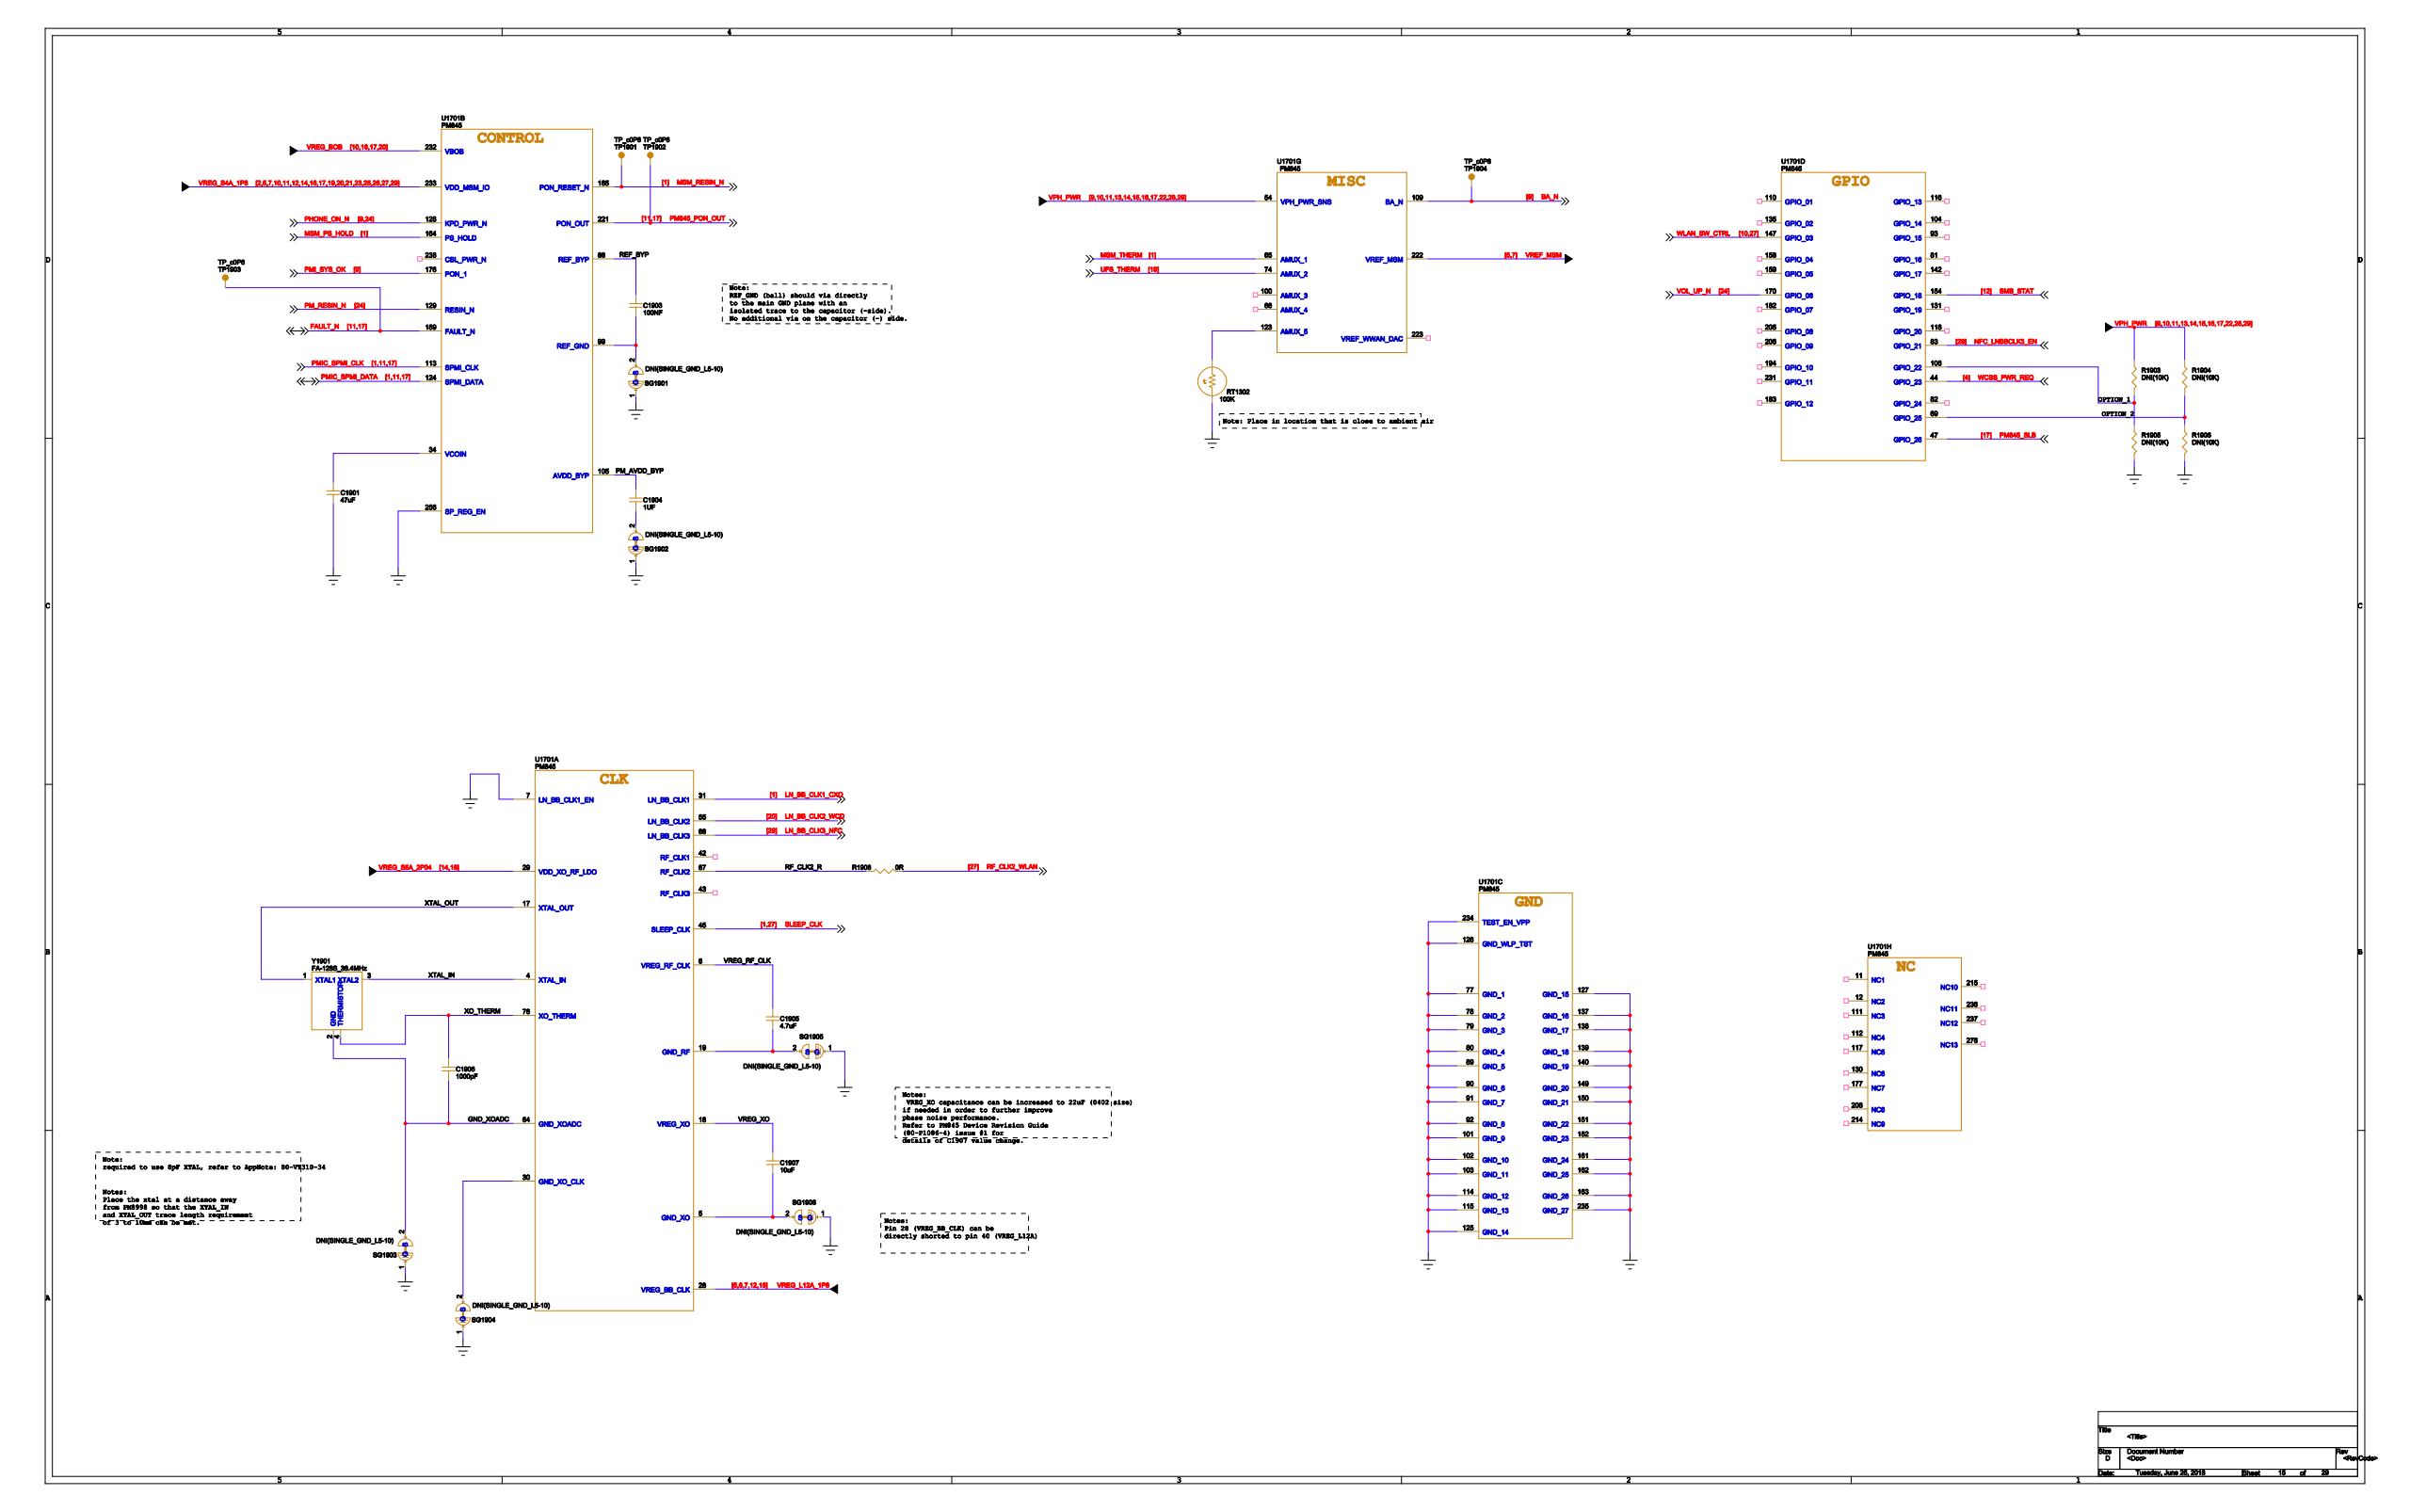Circuit board | Cadence Allegro | 802 parts | 566 nets | one sheet of the schematic
Parts on this sheet (reference | value | footprint):
C1901 | 47uF | C0805
C1903 | 100NF | C0201
C1904 | 1uF | C0201
C1905 | 4.7uF | 0402-BIG
C1906 | 1000pF | C0402
C1907 | 10uF | 0402-BIG_H0P9
R1903 | DNI(10K) | R0201
R1904 | DNI(10K) | R0201
R1905 | DNI(10K) | R0201
R1906 | DNI(10K) | R0201
R1908 | 0R | R0201
RT1302 | 100K | R0402
SG1901 | DNI(SINGLE_GND_L5-10) | GND_L5-10
SG1902 | DNI(SINGLE_GND_L5-10) | GND_L5-10
SG1903 | DNI(SINGLE_GND_L5-10) | GND_L5-10
SG1904 | DNI(SINGLE_GND_L5-10) | GND_L5-10
SG1905 | DNI(SINGLE_GND_L5-10) | GND_L5-10
SG1906 | DNI(SINGLE_GND_L5-10) | GND_L5-10
TP1901 | TP_c0P6 | TP_C0P6
TP1902 | TP_c0P6 | TP_C0P6
TP1903 | TP_c0P6 | TP_C0P6
TP1904 | TP_c0P6 | TP_C0P6
U1701 | PM845 | PM8998
Y1901 | FA-128S_38.4MHz | Y4_FA-128S_52MHZ
Nets of these parts (net: part-pin ...):
MSM_RESIN_N: TP1901-1 U1701-165
GND: C1901-2 R1905-2 R1906-2 RT1302-2 SG1901-1 SG1902-1 SG1903-1 SG1904-1 SG1905-1 SG1906-1 U1701-7 U1701-77 U1701-78 U1701-79 U1701-80 U1701-89 U1701-90 U1701-91 U1701-92 U1701-101 U1701-102 U1701-103 U1701-114 U1701-115 U1701-125 U1701-126 U1701-127 U1701-137 U1701-138 U1701-139 U1701-140 U1701-149 U1701-150 U1701-151 U1701-152 U1701-161 U1701-162 U1701-163 U1701-234 U1701-235 U1701-256
VREG_XO: C1907-1 U1701-18
N222387: C1907-2 SG1906-2 U1701-5
VPH_PWR: R1903-1 R1904-1 U1701-54
VREF_MSM: U1701-222
VREG_S4A_1P8: U1701-233
REF_BYP: C1903-1 U1701-88
N222581: C1903-2 SG1901-2 U1701-99
RF_CLK2_WLAN: R1908-2
LN_BB_CLK3_NFC: U1701-68
VREG_BOB: U1701-1 U1701-14 U1701-27 U1701-232
RF_CLK2_R: R1908-1 U1701-67
SMB_STAT: U1701-154
PM_AVDD_BYP: C1904-1 U1701-105
N222593: C1904-2 SG1902-2
VREG_L12A_1P8: U1701-28 U1701-40
VREG_S5A_2P04: U1701-29
N222535: C1901-1 U1701-34
VREG_RF_CLK: C1905-1 U1701-6
N221549: C1905-2 SG1905-2 U1701-19
XO_THERM: C1906-1 Y1901-4 U1701-76
GND_XOADC: C1906-2 SG1903-2 Y1901-2 U1701-64
N223236: R1903-2 R1905-1 U1701-106
N223248: R1904-2 R1906-1 U1701-69
VOL_UP_N: U1701-170
PM_RESIN_N: U1701-129
PHONE_ON_N: U1701-128
MSM_THERM: U1701-65
N222623: RT1302-1 U1701-123
UFS_THERM: U1701-74
N221111: SG1904-2 U1701-30
PM845_SLB: U1701-47
SLEEP_CLK: U1701-45
LN_BB_CLK1_CXO: U1701-31
MSM_PS_HOLD: U1701-164
PMIC_SPMI_DATA: U1701-124
PMIC_SPMI_CLK: U1701-113
PM845_PON_OUT: TP1902-1 U1701-221
FAULT_N: TP1903-1 U1701-189
BA_N: TP1904-1 U1701-109
LN_BB_CLK2_WCD: U1701-55
NFC_LNBBCLK3_EN: U1701-83
WCSS_PWR_REQ: U1701-44
PMI_SYS_OK: U1701-176
WLAN_SW_CTRL: U1701-147
XTAL_IN: Y1901-3 U1701-4
XTAL_OUT: Y1901-1 U1701-17